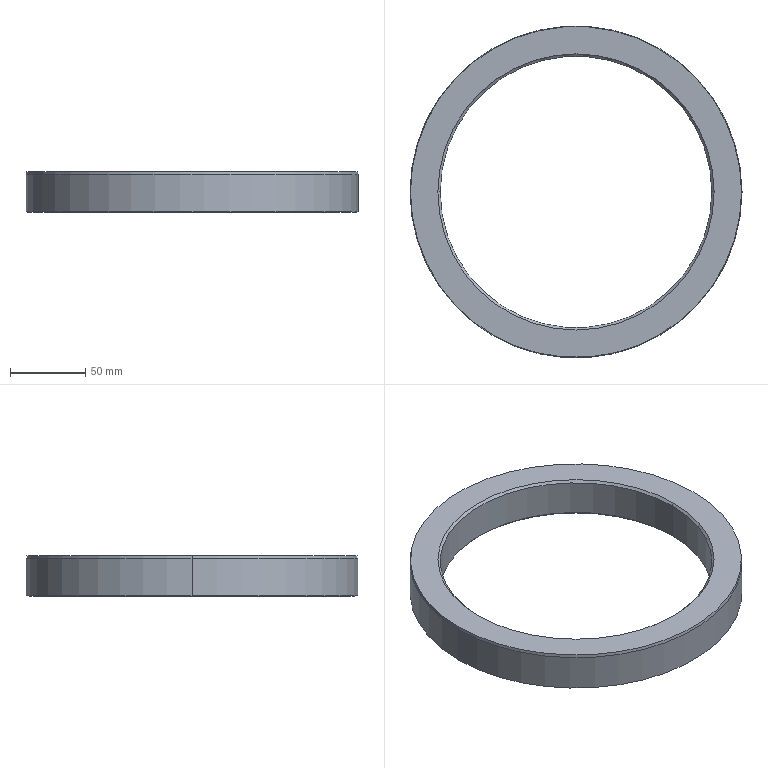Part | SolidWorks | features Chamfer 2, Extrusion 1 | 1 solid | 14 faces | box 220 x 220 x 27 mm | volume 337527 mm3 | cone 8 | cylinder 4 | plane 2 | commonest cylinder face diameters 180 x2 220 x2
STEP:
#1=CARTESIAN_POINT('',(-90.,0.,12.));
#2=VERTEX_POINT('',#1);
#3=CARTESIAN_POINT('',(90.,0.,12.));
#4=VERTEX_POINT('',#3);
#5=CARTESIAN_POINT('',(0.,0.,12.));
#6=DIRECTION('',(0.,0.,1.));
#7=DIRECTION('',(1.,0.,0.));
#8=AXIS2_PLACEMENT_3D('',#5,#6,#7);
#9=CIRCLE('',#8,90.);
#10=EDGE_CURVE('',#2,#4,#9,.T.);
#11=ORIENTED_EDGE('',*,*,#10,.F.);
#12=CARTESIAN_POINT('',(-91.5,0.,13.5));
#13=VERTEX_POINT('',#12);
#14=CARTESIAN_POINT('',(-90.,0.,12.));
#15=DIRECTION('',(-0.7071,0.,0.7071));
#16=VECTOR('',#15,1000.);
#17=LINE('',#14,#16);
#18=EDGE_CURVE('',#2,#13,#17,.T.);
#19=ORIENTED_EDGE('',*,*,#18,.T.);
#20=CARTESIAN_POINT('',(91.5,0.,13.5));
#21=VERTEX_POINT('',#20);
#22=CARTESIAN_POINT('',(0.,0.,13.5));
#23=DIRECTION('',(0.,0.,-1.));
#24=DIRECTION('',(1.,0.,0.));
#25=AXIS2_PLACEMENT_3D('',#22,#23,#24);
#26=CIRCLE('',#25,91.5);
#27=EDGE_CURVE('',#21,#13,#26,.T.);
#28=ORIENTED_EDGE('',*,*,#27,.F.);
#29=CARTESIAN_POINT('',(90.,0.,12.));
#30=DIRECTION('',(0.7071,0.,0.7071));
#31=VECTOR('',#30,1000.);
#32=LINE('',#29,#31);
#33=EDGE_CURVE('',#4,#21,#32,.T.);
#34=ORIENTED_EDGE('',*,*,#33,.F.);
#35=EDGE_LOOP('',(#11,#19,#28,#34));
#36=FACE_OUTER_BOUND('',#35,.T.);
#37=CARTESIAN_POINT('',(0.,0.,12.));
#38=DIRECTION('',(0.,0.,1.));
#39=DIRECTION('',(1.,0.,0.));
#40=AXIS2_PLACEMENT_3D('',#37,#38,#39);
#41=CONICAL_SURFACE('',#40,90.,0.7854);
#42=ADVANCED_FACE('',(#36),#41,.F.);
#43=CARTESIAN_POINT('',(90.,0.,-12.));
#44=VERTEX_POINT('',#43);
#45=CARTESIAN_POINT('',(-90.,0.,-12.));
#46=VERTEX_POINT('',#45);
#47=CARTESIAN_POINT('',(0.,0.,-12.));
#48=DIRECTION('',(0.,0.,-1.));
#49=DIRECTION('',(1.,0.,0.));
#50=AXIS2_PLACEMENT_3D('',#47,#48,#49);
#51=CIRCLE('',#50,90.);
#52=EDGE_CURVE('',#44,#46,#51,.T.);
#53=ORIENTED_EDGE('',*,*,#52,.F.);
#54=CARTESIAN_POINT('',(91.5,0.,-13.5));
#55=VERTEX_POINT('',#54);
#56=CARTESIAN_POINT('',(91.5,0.,-13.5));
#57=DIRECTION('',(0.7071,0.,-0.7071));
#58=VECTOR('',#57,1000.);
#59=LINE('',#56,#58);
#60=EDGE_CURVE('',#44,#55,#59,.T.);
#61=ORIENTED_EDGE('',*,*,#60,.T.);
#62=CARTESIAN_POINT('',(-91.5,0.,-13.5));
#63=VERTEX_POINT('',#62);
#64=CARTESIAN_POINT('',(0.,0.,-13.5));
#65=DIRECTION('',(0.,0.,1.));
#66=DIRECTION('',(1.,0.,0.));
#67=AXIS2_PLACEMENT_3D('',#64,#65,#66);
#68=CIRCLE('',#67,91.5);
#69=EDGE_CURVE('',#63,#55,#68,.T.);
#70=ORIENTED_EDGE('',*,*,#69,.F.);
#71=CARTESIAN_POINT('',(-91.5,0.,-13.5));
#72=DIRECTION('',(-0.7071,0.,-0.7071));
#73=VECTOR('',#72,1000.);
#74=LINE('',#71,#73);
#75=EDGE_CURVE('',#46,#63,#74,.T.);
#76=ORIENTED_EDGE('',*,*,#75,.F.);
#77=EDGE_LOOP('',(#53,#61,#70,#76));
#78=FACE_OUTER_BOUND('',#77,.T.);
#79=CARTESIAN_POINT('',(0.,0.,-13.5));
#80=DIRECTION('',(0.,0.,-1.));
#81=DIRECTION('',(-1.,0.,0.));
#82=AXIS2_PLACEMENT_3D('',#79,#80,#81);
#83=CONICAL_SURFACE('',#82,91.5,0.7854);
#84=ADVANCED_FACE('',(#78),#83,.F.);
#85=CARTESIAN_POINT('',(109.647,0.,13.5));
#86=VERTEX_POINT('',#85);
#87=CARTESIAN_POINT('',(-109.647,0.,13.5));
#88=VERTEX_POINT('',#87);
#89=CARTESIAN_POINT('',(0.,0.,13.5));
#90=DIRECTION('',(0.,0.,1.));
#91=DIRECTION('',(1.,0.,0.));
#92=AXIS2_PLACEMENT_3D('',#89,#90,#91);
#93=CIRCLE('',#92,109.647);
#94=EDGE_CURVE('',#86,#88,#93,.T.);
#95=ORIENTED_EDGE('',*,*,#94,.F.);
#96=CARTESIAN_POINT('',(110.,0.,11.5));
#97=VERTEX_POINT('',#96);
#98=CARTESIAN_POINT('',(109.647,0.,13.5));
#99=DIRECTION('',(0.1736,0.,-0.9848));
#100=VECTOR('',#99,1000.);
#101=LINE('',#98,#100);
#102=EDGE_CURVE('',#86,#97,#101,.T.);
#103=ORIENTED_EDGE('',*,*,#102,.T.);
#104=CARTESIAN_POINT('',(-110.,0.,11.5));
#105=VERTEX_POINT('',#104);
#106=CARTESIAN_POINT('',(0.,0.,11.5));
#107=DIRECTION('',(0.,0.,-1.));
#108=DIRECTION('',(1.,0.,0.));
#109=AXIS2_PLACEMENT_3D('',#106,#107,#108);
#110=CIRCLE('',#109,110.);
#111=EDGE_CURVE('',#105,#97,#110,.T.);
#112=ORIENTED_EDGE('',*,*,#111,.F.);
#113=CARTESIAN_POINT('',(-109.647,0.,13.5));
#114=DIRECTION('',(-0.1736,0.,-0.9848));
#115=VECTOR('',#114,1000.);
#116=LINE('',#113,#115);
#117=EDGE_CURVE('',#88,#105,#116,.T.);
#118=ORIENTED_EDGE('',*,*,#117,.F.);
#119=EDGE_LOOP('',(#95,#103,#112,#118));
#120=FACE_OUTER_BOUND('',#119,.T.);
#121=CARTESIAN_POINT('',(0.,0.,13.5));
#122=DIRECTION('',(0.,0.,-1.));
#123=DIRECTION('',(-1.,0.,0.));
#124=AXIS2_PLACEMENT_3D('',#121,#122,#123);
#125=CONICAL_SURFACE('',#124,109.647,0.1745);
#126=ADVANCED_FACE('',(#120),#125,.T.);
#127=CARTESIAN_POINT('',(-108.,0.,-13.5));
#128=VERTEX_POINT('',#127);
#129=CARTESIAN_POINT('',(108.,0.,-13.5));
#130=VERTEX_POINT('',#129);
#131=CARTESIAN_POINT('',(0.,0.,-13.5));
#132=DIRECTION('',(0.,0.,-1.));
#133=DIRECTION('',(1.,0.,0.));
#134=AXIS2_PLACEMENT_3D('',#131,#132,#133);
#135=CIRCLE('',#134,108.);
#136=EDGE_CURVE('',#128,#130,#135,.T.);
#137=ORIENTED_EDGE('',*,*,#136,.F.);
#138=CARTESIAN_POINT('',(-110.,0.,-13.147));
#139=VERTEX_POINT('',#138);
#140=CARTESIAN_POINT('',(-110.,0.,-13.147));
#141=DIRECTION('',(-0.9848,0.,0.1736));
#142=VECTOR('',#141,1000.);
#143=LINE('',#140,#142);
#144=EDGE_CURVE('',#128,#139,#143,.T.);
#145=ORIENTED_EDGE('',*,*,#144,.T.);
#146=CARTESIAN_POINT('',(110.,0.,-13.147));
#147=VERTEX_POINT('',#146);
#148=CARTESIAN_POINT('',(0.,0.,-13.147));
#149=DIRECTION('',(0.,0.,1.));
#150=DIRECTION('',(1.,0.,0.));
#151=AXIS2_PLACEMENT_3D('',#148,#149,#150);
#152=CIRCLE('',#151,110.);
#153=EDGE_CURVE('',#147,#139,#152,.T.);
#154=ORIENTED_EDGE('',*,*,#153,.F.);
#155=CARTESIAN_POINT('',(110.,0.,-13.147));
#156=DIRECTION('',(0.9848,0.,0.1736));
#157=VECTOR('',#156,1000.);
#158=LINE('',#155,#157);
#159=EDGE_CURVE('',#130,#147,#158,.T.);
#160=ORIENTED_EDGE('',*,*,#159,.F.);
#161=EDGE_LOOP('',(#137,#145,#154,#160));
#162=FACE_OUTER_BOUND('',#161,.T.);
#163=CARTESIAN_POINT('',(0.,0.,-13.147));
#164=DIRECTION('',(0.,0.,1.));
#165=DIRECTION('',(1.,0.,0.));
#166=AXIS2_PLACEMENT_3D('',#163,#164,#165);
#167=CONICAL_SURFACE('',#166,110.,1.396);
#168=ADVANCED_FACE('',(#162),#167,.T.);
#169=ORIENTED_EDGE('',*,*,#10,.T.);
#170=CARTESIAN_POINT('',(90.,0.,13.5));
#171=DIRECTION('',(0.,0.,-1.));
#172=VECTOR('',#171,1000.);
#173=LINE('',#170,#172);
#174=EDGE_CURVE('',#4,#44,#173,.T.);
#175=ORIENTED_EDGE('',*,*,#174,.T.);
#176=ORIENTED_EDGE('',*,*,#52,.T.);
#177=CARTESIAN_POINT('',(-90.,0.,13.5));
#178=DIRECTION('',(0.,0.,-1.));
#179=VECTOR('',#178,1000.);
#180=LINE('',#177,#179);
#181=EDGE_CURVE('',#2,#46,#180,.T.);
#182=ORIENTED_EDGE('',*,*,#181,.F.);
#183=EDGE_LOOP('',(#169,#175,#176,#182));
#184=FACE_OUTER_BOUND('',#183,.T.);
#185=CARTESIAN_POINT('',(0.,0.,13.5));
#186=DIRECTION('',(0.,0.,-1.));
#187=DIRECTION('',(-1.,0.,0.));
#188=AXIS2_PLACEMENT_3D('',#185,#186,#187);
#189=CYLINDRICAL_SURFACE('',#188,90.);
#190=ADVANCED_FACE('',(#184),#189,.F.);
#191=ORIENTED_EDGE('',*,*,#111,.T.);
#192=CARTESIAN_POINT('',(110.,0.,13.5));
#193=DIRECTION('',(0.,0.,-1.));
#194=VECTOR('',#193,1000.);
#195=LINE('',#192,#194);
#196=EDGE_CURVE('',#97,#147,#195,.T.);
#197=ORIENTED_EDGE('',*,*,#196,.T.);
#198=ORIENTED_EDGE('',*,*,#153,.T.);
#199=CARTESIAN_POINT('',(-110.,0.,13.5));
#200=DIRECTION('',(0.,0.,-1.));
#201=VECTOR('',#200,1000.);
#202=LINE('',#199,#201);
#203=EDGE_CURVE('',#105,#139,#202,.T.);
#204=ORIENTED_EDGE('',*,*,#203,.F.);
#205=EDGE_LOOP('',(#191,#197,#198,#204));
#206=FACE_OUTER_BOUND('',#205,.T.);
#207=CARTESIAN_POINT('',(0.,0.,13.5));
#208=DIRECTION('',(0.,0.,-1.));
#209=DIRECTION('',(-1.,0.,0.));
#210=AXIS2_PLACEMENT_3D('',#207,#208,#209);
#211=CYLINDRICAL_SURFACE('',#210,110.);
#212=ADVANCED_FACE('',(#206),#211,.T.);
#213=ORIENTED_EDGE('',*,*,#27,.T.);
#214=CARTESIAN_POINT('',(0.,0.,13.5));
#215=DIRECTION('',(0.,0.,-1.));
#216=DIRECTION('',(1.,0.,0.));
#217=AXIS2_PLACEMENT_3D('',#214,#215,#216);
#218=CIRCLE('',#217,91.5);
#219=EDGE_CURVE('',#13,#21,#218,.T.);
#220=ORIENTED_EDGE('',*,*,#219,.T.);
#221=EDGE_LOOP('',(#213,#220));
#222=FACE_BOUND('',#221,.T.);
#223=CARTESIAN_POINT('',(0.,0.,13.5));
#224=DIRECTION('',(0.,0.,1.));
#225=DIRECTION('',(1.,0.,0.));
#226=AXIS2_PLACEMENT_3D('',#223,#224,#225);
#227=CIRCLE('',#226,109.647);
#228=EDGE_CURVE('',#88,#86,#227,.T.);
#229=ORIENTED_EDGE('',*,*,#228,.T.);
#230=ORIENTED_EDGE('',*,*,#94,.T.);
#231=EDGE_LOOP('',(#229,#230));
#232=FACE_OUTER_BOUND('',#231,.T.);
#233=CARTESIAN_POINT('',(0.,0.,13.5));
#234=DIRECTION('',(0.,0.,1.));
#235=DIRECTION('',(1.,0.,0.));
#236=AXIS2_PLACEMENT_3D('',#233,#234,#235);
#237=PLANE('',#236);
#238=ADVANCED_FACE('',(#222,#232),#237,.T.);
#239=ORIENTED_EDGE('',*,*,#69,.T.);
#240=CARTESIAN_POINT('',(0.,0.,-13.5));
#241=DIRECTION('',(0.,0.,1.));
#242=DIRECTION('',(1.,0.,0.));
#243=AXIS2_PLACEMENT_3D('',#240,#241,#242);
#244=CIRCLE('',#243,91.5);
#245=EDGE_CURVE('',#55,#63,#244,.T.);
#246=ORIENTED_EDGE('',*,*,#245,.T.);
#247=EDGE_LOOP('',(#239,#246));
#248=FACE_BOUND('',#247,.T.);
#249=CARTESIAN_POINT('',(0.,0.,-13.5));
#250=DIRECTION('',(0.,0.,-1.));
#251=DIRECTION('',(1.,0.,0.));
#252=AXIS2_PLACEMENT_3D('',#249,#250,#251);
#253=CIRCLE('',#252,108.);
#254=EDGE_CURVE('',#130,#128,#253,.T.);
#255=ORIENTED_EDGE('',*,*,#254,.T.);
#256=ORIENTED_EDGE('',*,*,#136,.T.);
#257=EDGE_LOOP('',(#255,#256));
#258=FACE_OUTER_BOUND('',#257,.T.);
#259=CARTESIAN_POINT('',(0.,0.,-13.5));
#260=DIRECTION('',(0.,0.,1.));
#261=DIRECTION('',(1.,0.,0.));
#262=AXIS2_PLACEMENT_3D('',#259,#260,#261);
#263=PLANE('',#262);
#264=ADVANCED_FACE('',(#248,#258),#263,.F.);
#265=ORIENTED_EDGE('',*,*,#196,.F.);
#266=CARTESIAN_POINT('',(0.,0.,11.5));
#267=DIRECTION('',(0.,0.,-1.));
#268=DIRECTION('',(1.,0.,0.));
#269=AXIS2_PLACEMENT_3D('',#266,#267,#268);
#270=CIRCLE('',#269,110.);
#271=EDGE_CURVE('',#97,#105,#270,.T.);
#272=ORIENTED_EDGE('',*,*,#271,.T.);
#273=ORIENTED_EDGE('',*,*,#203,.T.);
#274=CARTESIAN_POINT('',(0.,0.,-13.147));
#275=DIRECTION('',(0.,0.,1.));
#276=DIRECTION('',(1.,0.,0.));
#277=AXIS2_PLACEMENT_3D('',#274,#275,#276);
#278=CIRCLE('',#277,110.);
#279=EDGE_CURVE('',#139,#147,#278,.T.);
#280=ORIENTED_EDGE('',*,*,#279,.T.);
#281=EDGE_LOOP('',(#265,#272,#273,#280));
#282=FACE_OUTER_BOUND('',#281,.T.);
#283=CARTESIAN_POINT('',(0.,0.,13.5));
#284=DIRECTION('',(0.,0.,-1.));
#285=DIRECTION('',(-1.,0.,0.));
#286=AXIS2_PLACEMENT_3D('',#283,#284,#285);
#287=CYLINDRICAL_SURFACE('',#286,110.);
#288=ADVANCED_FACE('',(#282),#287,.T.);
#289=ORIENTED_EDGE('',*,*,#174,.F.);
#290=CARTESIAN_POINT('',(0.,0.,12.));
#291=DIRECTION('',(0.,0.,1.));
#292=DIRECTION('',(1.,0.,0.));
#293=AXIS2_PLACEMENT_3D('',#290,#291,#292);
#294=CIRCLE('',#293,90.);
#295=EDGE_CURVE('',#4,#2,#294,.T.);
#296=ORIENTED_EDGE('',*,*,#295,.T.);
#297=ORIENTED_EDGE('',*,*,#181,.T.);
#298=CARTESIAN_POINT('',(0.,0.,-12.));
#299=DIRECTION('',(0.,0.,-1.));
#300=DIRECTION('',(1.,0.,0.));
#301=AXIS2_PLACEMENT_3D('',#298,#299,#300);
#302=CIRCLE('',#301,90.);
#303=EDGE_CURVE('',#46,#44,#302,.T.);
#304=ORIENTED_EDGE('',*,*,#303,.T.);
#305=EDGE_LOOP('',(#289,#296,#297,#304));
#306=FACE_OUTER_BOUND('',#305,.T.);
#307=CARTESIAN_POINT('',(0.,0.,13.5));
#308=DIRECTION('',(0.,0.,-1.));
#309=DIRECTION('',(-1.,0.,0.));
#310=AXIS2_PLACEMENT_3D('',#307,#308,#309);
#311=CYLINDRICAL_SURFACE('',#310,90.);
#312=ADVANCED_FACE('',(#306),#311,.F.);
#313=ORIENTED_EDGE('',*,*,#144,.F.);
#314=ORIENTED_EDGE('',*,*,#254,.F.);
#315=ORIENTED_EDGE('',*,*,#159,.T.);
#316=ORIENTED_EDGE('',*,*,#279,.F.);
#317=EDGE_LOOP('',(#313,#314,#315,#316));
#318=FACE_OUTER_BOUND('',#317,.T.);
#319=CARTESIAN_POINT('',(0.,0.,-13.147));
#320=DIRECTION('',(0.,0.,1.));
#321=DIRECTION('',(1.,0.,0.));
#322=AXIS2_PLACEMENT_3D('',#319,#320,#321);
#323=CONICAL_SURFACE('',#322,110.,1.396);
#324=ADVANCED_FACE('',(#318),#323,.T.);
#325=ORIENTED_EDGE('',*,*,#102,.F.);
#326=ORIENTED_EDGE('',*,*,#228,.F.);
#327=ORIENTED_EDGE('',*,*,#117,.T.);
#328=ORIENTED_EDGE('',*,*,#271,.F.);
#329=EDGE_LOOP('',(#325,#326,#327,#328));
#330=FACE_OUTER_BOUND('',#329,.T.);
#331=CARTESIAN_POINT('',(0.,0.,13.5));
#332=DIRECTION('',(0.,0.,-1.));
#333=DIRECTION('',(-1.,0.,0.));
#334=AXIS2_PLACEMENT_3D('',#331,#332,#333);
#335=CONICAL_SURFACE('',#334,109.647,0.1745);
#336=ADVANCED_FACE('',(#330),#335,.T.);
#337=ORIENTED_EDGE('',*,*,#60,.F.);
#338=ORIENTED_EDGE('',*,*,#303,.F.);
#339=ORIENTED_EDGE('',*,*,#75,.T.);
#340=ORIENTED_EDGE('',*,*,#245,.F.);
#341=EDGE_LOOP('',(#337,#338,#339,#340));
#342=FACE_OUTER_BOUND('',#341,.T.);
#343=CARTESIAN_POINT('',(0.,0.,-13.5));
#344=DIRECTION('',(0.,0.,-1.));
#345=DIRECTION('',(-1.,0.,0.));
#346=AXIS2_PLACEMENT_3D('',#343,#344,#345);
#347=CONICAL_SURFACE('',#346,91.5,0.7854);
#348=ADVANCED_FACE('',(#342),#347,.F.);
#349=ORIENTED_EDGE('',*,*,#18,.F.);
#350=ORIENTED_EDGE('',*,*,#295,.F.);
#351=ORIENTED_EDGE('',*,*,#33,.T.);
#352=ORIENTED_EDGE('',*,*,#219,.F.);
#353=EDGE_LOOP('',(#349,#350,#351,#352));
#354=FACE_OUTER_BOUND('',#353,.T.);
#355=CARTESIAN_POINT('',(0.,0.,12.));
#356=DIRECTION('',(0.,0.,1.));
#357=DIRECTION('',(1.,0.,0.));
#358=AXIS2_PLACEMENT_3D('',#355,#356,#357);
#359=CONICAL_SURFACE('',#358,90.,0.7854);
#360=ADVANCED_FACE('',(#354),#359,.F.);
#361=CLOSED_SHELL('',(#42,#84,#126,#168,#190,#212,#238,#264,#288,#312,#324,#336,#348,#360));
#362=MANIFOLD_SOLID_BREP('',#361);
#363=CARTESIAN_POINT('',(0.,0.,0.));
#364=DIRECTION('',(0.,0.,1.));
#365=DIRECTION('',(1.,0.,0.));
#366=AXIS2_PLACEMENT_3D('',#363,#364,#365);
#367=(LENGTH_UNIT()NAMED_UNIT(*)SI_UNIT(.MILLI.,.METRE.));
#368=UNCERTAINTY_MEASURE_WITH_UNIT(LENGTH_MEASURE(0.00001),#367,'','');
#369=(NAMED_UNIT(*)PLANE_ANGLE_UNIT()SI_UNIT($,.RADIAN.));
#370=(NAMED_UNIT(*)SI_UNIT($,.STERADIAN.)SOLID_ANGLE_UNIT());
#371=(GEOMETRIC_REPRESENTATION_CONTEXT(3)GLOBAL_UNCERTAINTY_ASSIGNED_CONTEXT((#368))GLOBAL_UNIT_ASSIGNED_CONTEXT((#367,#369,#370))REPRESENTATION_CONTEXT('',''));
#372=ADVANCED_BREP_SHAPE_REPRESENTATION('',(#362,#366),#371);